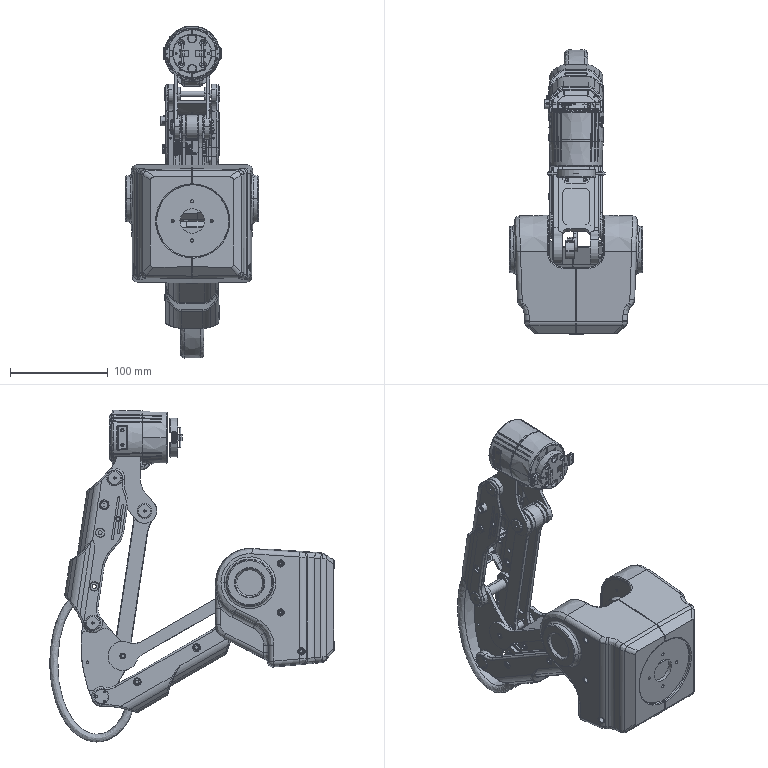Part | NX | features BREP 245, REPLACE_FACE 5, DATUM_CSYS 4, SKETCH 4, DELETE FACE 3, Delete Body 2, EXTRUDE 2, UNITE 1 | 263 solids | 7718 faces | volume 823065 mm3 | plane 3214 | cylinder 2698 | spline 923 | cone 462 | torus 248 | sphere 173 | commonest cylinder face diameters 1 x256 2 x220 10 x148 4 x135 2.5 x104 0.1 x102